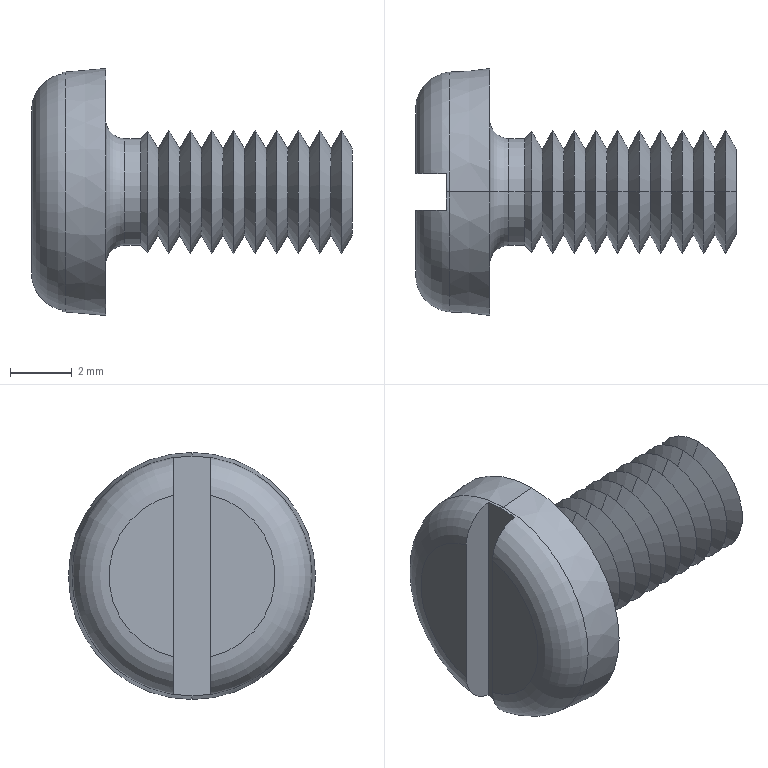Part | SolidWorks | features Cut 1, LPattern 1, RevCut 1, Revolution 1 | 1 solid | 55 faces | box 10.4 x 8 x 8 mm | volume 174.956 mm3 | cone 42 | plane 7 | torus 4 | cylinder 2 | commonest cylinder face diameters 3.464 x2
STEP:
#1=CARTESIAN_POINT('',(3.532,0.,1.732));
#2=VERTEX_POINT('',#1);
#3=CARTESIAN_POINT('',(3.532,0.,-1.732));
#4=VERTEX_POINT('',#3);
#5=CARTESIAN_POINT('',(3.532,0.,0.));
#6=DIRECTION('',(-1.,0.,0.));
#7=DIRECTION('',(0.,0.,1.));
#8=AXIS2_PLACEMENT_3D('',#5,#6,#7);
#9=CIRCLE('',#8,1.732);
#10=EDGE_CURVE('',#2,#4,#9,.T.);
#11=ORIENTED_EDGE('',*,*,#10,.F.);
#12=CARTESIAN_POINT('',(3.766,0.,1.966));
#13=VERTEX_POINT('',#12);
#14=CARTESIAN_POINT('',(3.8,0.,2.));
#15=DIRECTION('',(0.7071,0.,0.7071));
#16=VECTOR('',#15,1000.);
#17=LINE('',#14,#16);
#18=EDGE_CURVE('',#2,#13,#17,.T.);
#19=ORIENTED_EDGE('',*,*,#18,.T.);
#20=CARTESIAN_POINT('',(3.766,0.,-1.966));
#21=VERTEX_POINT('',#20);
#22=CARTESIAN_POINT('',(3.766,0.,0.));
#23=DIRECTION('',(-1.,0.,0.));
#24=DIRECTION('',(0.,0.,1.));
#25=AXIS2_PLACEMENT_3D('',#22,#23,#24);
#26=CIRCLE('',#25,1.966);
#27=EDGE_CURVE('',#13,#21,#26,.T.);
#28=ORIENTED_EDGE('',*,*,#27,.T.);
#29=CARTESIAN_POINT('',(3.8,0.,-2.));
#30=DIRECTION('',(0.7071,0.,-0.7071));
#31=VECTOR('',#30,1000.);
#32=LINE('',#29,#31);
#33=EDGE_CURVE('',#4,#21,#32,.T.);
#34=ORIENTED_EDGE('',*,*,#33,.F.);
#35=EDGE_LOOP('',(#11,#19,#28,#34));
#36=FACE_OUTER_BOUND('',#35,.T.);
#37=CARTESIAN_POINT('',(3.8,0.,0.));
#38=DIRECTION('',(1.,0.,0.));
#39=DIRECTION('',(0.,0.,-1.));
#40=AXIS2_PLACEMENT_3D('',#37,#38,#39);
#41=CONICAL_SURFACE('',#40,2.,0.7854);
#42=ADVANCED_FACE('',(#36),#41,.T.);
#43=ORIENTED_EDGE('',*,*,#10,.T.);
#44=CARTESIAN_POINT('',(3.018,0.,-1.732));
#45=VERTEX_POINT('',#44);
#46=CARTESIAN_POINT('',(-2.477,0.,-1.732));
#47=DIRECTION('',(-1.,0.,0.));
#48=VECTOR('',#47,1000.);
#49=LINE('',#46,#48);
#50=EDGE_CURVE('',#4,#45,#49,.T.);
#51=ORIENTED_EDGE('',*,*,#50,.T.);
#52=CARTESIAN_POINT('',(3.018,0.,1.732));
#53=VERTEX_POINT('',#52);
#54=CARTESIAN_POINT('',(3.018,0.,0.));
#55=DIRECTION('',(-1.,0.,0.));
#56=DIRECTION('',(0.,0.,1.));
#57=AXIS2_PLACEMENT_3D('',#54,#55,#56);
#58=CIRCLE('',#57,1.732);
#59=EDGE_CURVE('',#53,#45,#58,.T.);
#60=ORIENTED_EDGE('',*,*,#59,.F.);
#61=CARTESIAN_POINT('',(-2.477,0.,1.732));
#62=DIRECTION('',(-1.,0.,0.));
#63=VECTOR('',#62,1000.);
#64=LINE('',#61,#63);
#65=EDGE_CURVE('',#2,#53,#64,.T.);
#66=ORIENTED_EDGE('',*,*,#65,.F.);
#67=EDGE_LOOP('',(#43,#51,#60,#66));
#68=FACE_OUTER_BOUND('',#67,.T.);
#69=CARTESIAN_POINT('',(-2.477,0.,0.));
#70=DIRECTION('',(-1.,0.,0.));
#71=DIRECTION('',(0.,0.,1.));
#72=AXIS2_PLACEMENT_3D('',#69,#70,#71);
#73=CYLINDRICAL_SURFACE('',#72,1.732);
#74=ADVANCED_FACE('',(#68),#73,.T.);
#75=CARTESIAN_POINT('',(2.4,0.,-2.35));
#76=VERTEX_POINT('',#75);
#77=CARTESIAN_POINT('',(2.4,0.,2.35));
#78=VERTEX_POINT('',#77);
#79=CARTESIAN_POINT('',(2.4,0.,0.));
#80=DIRECTION('',(-1.,0.,0.));
#81=DIRECTION('',(0.,0.,1.));
#82=AXIS2_PLACEMENT_3D('',#79,#80,#81);
#83=CIRCLE('',#82,2.35);
#84=EDGE_CURVE('',#76,#78,#83,.T.);
#85=ORIENTED_EDGE('',*,*,#84,.F.);
#86=CARTESIAN_POINT('',(3.018,0.,-2.35));
#87=DIRECTION('',(0.,1.,0.));
#88=DIRECTION('',(0.,0.,1.));
#89=AXIS2_PLACEMENT_3D('',#86,#87,#88);
#90=CIRCLE('',#89,0.618);
#91=EDGE_CURVE('',#76,#45,#90,.T.);
#92=ORIENTED_EDGE('',*,*,#91,.T.);
#93=CARTESIAN_POINT('',(3.018,0.,0.));
#94=DIRECTION('',(-1.,0.,0.));
#95=DIRECTION('',(0.,0.,1.));
#96=AXIS2_PLACEMENT_3D('',#93,#94,#95);
#97=CIRCLE('',#96,1.732);
#98=EDGE_CURVE('',#45,#53,#97,.T.);
#99=ORIENTED_EDGE('',*,*,#98,.T.);
#100=CARTESIAN_POINT('',(3.018,0.,2.35));
#101=DIRECTION('',(0.,-1.,0.));
#102=DIRECTION('',(0.,0.,-1.));
#103=AXIS2_PLACEMENT_3D('',#100,#101,#102);
#104=CIRCLE('',#103,0.618);
#105=EDGE_CURVE('',#78,#53,#104,.T.);
#106=ORIENTED_EDGE('',*,*,#105,.F.);
#107=EDGE_LOOP('',(#85,#92,#99,#106));
#108=FACE_OUTER_BOUND('',#107,.T.);
#109=CARTESIAN_POINT('',(3.018,0.,0.));
#110=DIRECTION('',(-1.,0.,0.));
#111=DIRECTION('',(0.,0.,1.));
#112=AXIS2_PLACEMENT_3D('',#109,#110,#111);
#113=TOROIDAL_SURFACE('',#112,2.35,0.618);
#114=ADVANCED_FACE('',(#108),#113,.F.);
#115=CARTESIAN_POINT('',(1.095,0.,3.886));
#116=VERTEX_POINT('',#115);
#117=CARTESIAN_POINT('',(1.095,0.,-3.886));
#118=VERTEX_POINT('',#117);
#119=CARTESIAN_POINT('',(1.095,0.,0.));
#120=DIRECTION('',(-1.,0.,0.));
#121=DIRECTION('',(0.,0.,1.));
#122=AXIS2_PLACEMENT_3D('',#119,#120,#121);
#123=CIRCLE('',#122,3.886);
#124=EDGE_CURVE('',#116,#118,#123,.T.);
#125=ORIENTED_EDGE('',*,*,#124,.F.);
#126=CARTESIAN_POINT('',(2.4,0.,4.));
#127=VERTEX_POINT('',#126);
#128=CARTESIAN_POINT('',(2.4,0.,4.));
#129=DIRECTION('',(0.9962,0.,0.08716));
#130=VECTOR('',#129,1000.);
#131=LINE('',#128,#130);
#132=EDGE_CURVE('',#116,#127,#131,.T.);
#133=ORIENTED_EDGE('',*,*,#132,.T.);
#134=CARTESIAN_POINT('',(2.4,0.,-4.));
#135=VERTEX_POINT('',#134);
#136=CARTESIAN_POINT('',(2.4,0.,0.));
#137=DIRECTION('',(-1.,0.,0.));
#138=DIRECTION('',(0.,0.,1.));
#139=AXIS2_PLACEMENT_3D('',#136,#137,#138);
#140=CIRCLE('',#139,4.);
#141=EDGE_CURVE('',#127,#135,#140,.T.);
#142=ORIENTED_EDGE('',*,*,#141,.T.);
#143=CARTESIAN_POINT('',(2.4,0.,-4.));
#144=DIRECTION('',(0.9962,0.,-0.08716));
#145=VECTOR('',#144,1000.);
#146=LINE('',#143,#145);
#147=EDGE_CURVE('',#118,#135,#146,.T.);
#148=ORIENTED_EDGE('',*,*,#147,.F.);
#149=EDGE_LOOP('',(#125,#133,#142,#148));
#150=FACE_OUTER_BOUND('',#149,.T.);
#151=CARTESIAN_POINT('',(2.4,0.,0.));
#152=DIRECTION('',(1.,0.,0.));
#153=DIRECTION('',(0.,0.,-1.));
#154=AXIS2_PLACEMENT_3D('',#151,#152,#153);
#155=CONICAL_SURFACE('',#154,4.,0.08727);
#156=ADVANCED_FACE('',(#150),#155,.T.);
#157=ORIENTED_EDGE('',*,*,#124,.T.);
#158=CARTESIAN_POINT('',(1.,0.,-3.874));
#159=VERTEX_POINT('',#158);
#160=CARTESIAN_POINT('',(1.2,0.,-2.69));
#161=DIRECTION('',(0.,1.,0.));
#162=DIRECTION('',(0.,0.,1.));
#163=AXIS2_PLACEMENT_3D('',#160,#161,#162);
#164=CIRCLE('',#163,1.2);
#165=EDGE_CURVE('',#118,#159,#164,.T.);
#166=ORIENTED_EDGE('',*,*,#165,.T.);
#167=CARTESIAN_POINT('',(1.,0.6,-3.827));
#168=VERTEX_POINT('',#167);
#169=CARTESIAN_POINT('',(1.,0.,0.));
#170=DIRECTION('',(1.,0.,0.));
#171=DIRECTION('',(0.,1.,0.));
#172=AXIS2_PLACEMENT_3D('',#169,#170,#171);
#173=CIRCLE('',#172,3.874);
#174=EDGE_CURVE('',#159,#168,#173,.T.);
#175=ORIENTED_EDGE('',*,*,#174,.T.);
#176=CARTESIAN_POINT('',(0.,0.6,-2.623));
#177=VERTEX_POINT('',#176);
#178=CARTESIAN_POINT('',(1.,0.6,-3.827));
#179=CARTESIAN_POINT('',(0.86,0.6,-3.803));
#180=CARTESIAN_POINT('',(0.7256,0.6,-3.754));
#181=CARTESIAN_POINT('',(0.4794,0.6,-3.611));
#182=CARTESIAN_POINT('',(0.3687,0.6,-3.516));
#183=CARTESIAN_POINT('',(0.1895,0.6,-3.298));
#184=CARTESIAN_POINT('',(0.1184,0.6,-3.172));
#185=CARTESIAN_POINT('',(0.02425,0.6,-2.906));
#186=CARTESIAN_POINT('',(0.,0.6,-2.764));
#187=CARTESIAN_POINT('',(0.,0.6,-2.623));
#188=B_SPLINE_CURVE_WITH_KNOTS('',3,(#178,#179,#180,#181,#182,#183,#184,#185,#186,#187),.UNSPECIFIED.,.F.,.F.,(4,2,2,2,4),(0.006929,0.007352,0.007774,0.008197,0.00862),.UNSPECIFIED.);
#189=EDGE_CURVE('',#168,#177,#188,.T.);
#190=ORIENTED_EDGE('',*,*,#189,.T.);
#191=CARTESIAN_POINT('',(0.,0.6,2.623));
#192=VERTEX_POINT('',#191);
#193=CARTESIAN_POINT('',(0.,0.,0.));
#194=DIRECTION('',(-1.,0.,0.));
#195=DIRECTION('',(0.,0.,1.));
#196=AXIS2_PLACEMENT_3D('',#193,#194,#195);
#197=CIRCLE('',#196,2.69);
#198=EDGE_CURVE('',#192,#177,#197,.T.);
#199=ORIENTED_EDGE('',*,*,#198,.F.);
#200=CARTESIAN_POINT('',(1.,0.6,3.827));
#201=VERTEX_POINT('',#200);
#202=CARTESIAN_POINT('',(0.,0.6,2.623));
#203=CARTESIAN_POINT('',(0.,0.6,2.908));
#204=CARTESIAN_POINT('',(0.09837,0.6,3.188));
#205=CARTESIAN_POINT('',(0.3703,0.6,3.518));
#206=CARTESIAN_POINT('',(0.4787,0.6,3.61));
#207=CARTESIAN_POINT('',(0.7255,0.6,3.754));
#208=CARTESIAN_POINT('',(0.8588,0.6,3.803));
#209=CARTESIAN_POINT('',(1.,0.6,3.827));
#210=B_SPLINE_CURVE_WITH_KNOTS('',3,(#202,#203,#204,#205,#206,#207,#208,#209),.UNSPECIFIED.,.F.,.F.,(4,2,2,4),(0.001251,0.002097,0.00252,0.002944),.UNSPECIFIED.);
#211=EDGE_CURVE('',#192,#201,#210,.T.);
#212=ORIENTED_EDGE('',*,*,#211,.T.);
#213=CARTESIAN_POINT('',(1.,0.,3.874));
#214=VERTEX_POINT('',#213);
#215=CARTESIAN_POINT('',(1.,0.,0.));
#216=DIRECTION('',(1.,0.,0.));
#217=DIRECTION('',(0.,1.,0.));
#218=AXIS2_PLACEMENT_3D('',#215,#216,#217);
#219=CIRCLE('',#218,3.874);
#220=EDGE_CURVE('',#201,#214,#219,.T.);
#221=ORIENTED_EDGE('',*,*,#220,.T.);
#222=CARTESIAN_POINT('',(1.2,0.,2.69));
#223=DIRECTION('',(0.,-1.,0.));
#224=DIRECTION('',(0.,0.,-1.));
#225=AXIS2_PLACEMENT_3D('',#222,#223,#224);
#226=CIRCLE('',#225,1.2);
#227=EDGE_CURVE('',#116,#214,#226,.T.);
#228=ORIENTED_EDGE('',*,*,#227,.F.);
#229=EDGE_LOOP('',(#157,#166,#175,#190,#199,#212,#221,#228));
#230=FACE_OUTER_BOUND('',#229,.T.);
#231=CARTESIAN_POINT('',(1.2,0.,0.));
#232=DIRECTION('',(-1.,0.,0.));
#233=DIRECTION('',(0.,0.,1.));
#234=AXIS2_PLACEMENT_3D('',#231,#232,#233);
#235=TOROIDAL_SURFACE('',#234,2.69,1.2);
#236=ADVANCED_FACE('',(#230),#235,.T.);
#237=CARTESIAN_POINT('',(4.1,0.,-1.394));
#238=VERTEX_POINT('',#237);
#239=CARTESIAN_POINT('',(4.1,0.,1.394));
#240=VERTEX_POINT('',#239);
#241=CARTESIAN_POINT('',(4.1,0.,0.));
#242=DIRECTION('',(1.,0.,0.));
#243=DIRECTION('',(0.,0.,-1.));
#244=AXIS2_PLACEMENT_3D('',#241,#242,#243);
#245=CIRCLE('',#244,1.394);
#246=EDGE_CURVE('',#238,#240,#245,.T.);
#247=ORIENTED_EDGE('',*,*,#246,.T.);
#248=CARTESIAN_POINT('',(4.446,0.,2.));
#249=VERTEX_POINT('',#248);
#250=CARTESIAN_POINT('',(4.1,0.,1.394));
#251=DIRECTION('',(0.4959,0.,0.8684));
#252=VECTOR('',#251,1000.);
#253=LINE('',#250,#252);
#254=EDGE_CURVE('',#240,#249,#253,.T.);
#255=ORIENTED_EDGE('',*,*,#254,.T.);
#256=CARTESIAN_POINT('',(4.446,0.,-2.));
#257=VERTEX_POINT('',#256);
#258=CARTESIAN_POINT('',(4.446,0.,0.));
#259=DIRECTION('',(1.,0.,0.));
#260=DIRECTION('',(0.,0.,-1.));
#261=AXIS2_PLACEMENT_3D('',#258,#259,#260);
#262=CIRCLE('',#261,2.);
#263=EDGE_CURVE('',#257,#249,#262,.T.);
#264=ORIENTED_EDGE('',*,*,#263,.F.);
#265=CARTESIAN_POINT('',(4.1,0.,-1.394));
#266=DIRECTION('',(0.4959,0.,-0.8684));
#267=VECTOR('',#266,1000.);
#268=LINE('',#265,#267);
#269=EDGE_CURVE('',#238,#257,#268,.T.);
#270=ORIENTED_EDGE('',*,*,#269,.F.);
#271=EDGE_LOOP('',(#247,#255,#264,#270));
#272=FACE_OUTER_BOUND('',#271,.T.);
#273=CARTESIAN_POINT('',(4.1,0.,0.));
#274=DIRECTION('',(1.,0.,0.));
#275=DIRECTION('',(0.,0.,-1.));
#276=AXIS2_PLACEMENT_3D('',#273,#274,#275);
#277=CONICAL_SURFACE('',#276,1.394,1.052);
#278=ADVANCED_FACE('',(#272),#277,.T.);
#279=ORIENTED_EDGE('',*,*,#246,.F.);
#280=CARTESIAN_POINT('',(3.746,0.,-2.));
#281=DIRECTION('',(-0.5041,0.,-0.8637));
#282=VECTOR('',#281,1000.);
#283=LINE('',#280,#282);
#284=EDGE_CURVE('',#238,#21,#283,.T.);
#285=ORIENTED_EDGE('',*,*,#284,.T.);
#286=ORIENTED_EDGE('',*,*,#27,.F.);
#287=CARTESIAN_POINT('',(3.746,0.,2.));
#288=DIRECTION('',(-0.5041,0.,0.8637));
#289=VECTOR('',#288,1000.);
#290=LINE('',#287,#289);
#291=EDGE_CURVE('',#240,#13,#290,.T.);
#292=ORIENTED_EDGE('',*,*,#291,.F.);
#293=EDGE_LOOP('',(#279,#285,#286,#292));
#294=FACE_OUTER_BOUND('',#293,.T.);
#295=CARTESIAN_POINT('',(3.746,0.,0.));
#296=DIRECTION('',(-1.,0.,0.));
#297=DIRECTION('',(0.,0.,1.));
#298=AXIS2_PLACEMENT_3D('',#295,#296,#297);
#299=CONICAL_SURFACE('',#298,2.,1.043);
#300=ADVANCED_FACE('',(#294),#299,.T.);
#301=CARTESIAN_POINT('',(4.8,0.,-1.394));
#302=VERTEX_POINT('',#301);
#303=CARTESIAN_POINT('',(4.8,0.,1.394));
#304=VERTEX_POINT('',#303);
#305=CARTESIAN_POINT('',(4.8,0.,0.));
#306=DIRECTION('',(1.,0.,0.));
#307=DIRECTION('',(0.,0.,-1.));
#308=AXIS2_PLACEMENT_3D('',#305,#306,#307);
#309=CIRCLE('',#308,1.394);
#310=EDGE_CURVE('',#302,#304,#309,.T.);
#311=ORIENTED_EDGE('',*,*,#310,.T.);
#312=CARTESIAN_POINT('',(5.146,0.,2.));
#313=VERTEX_POINT('',#312);
#314=CARTESIAN_POINT('',(4.8,0.,1.394));
#315=DIRECTION('',(0.4959,0.,0.8684));
#316=VECTOR('',#315,1000.);
#317=LINE('',#314,#316);
#318=EDGE_CURVE('',#304,#313,#317,.T.);
#319=ORIENTED_EDGE('',*,*,#318,.T.);
#320=CARTESIAN_POINT('',(5.146,0.,-2.));
#321=VERTEX_POINT('',#320);
#322=CARTESIAN_POINT('',(5.146,0.,0.));
#323=DIRECTION('',(1.,0.,0.));
#324=DIRECTION('',(0.,0.,-1.));
#325=AXIS2_PLACEMENT_3D('',#322,#323,#324);
#326=CIRCLE('',#325,2.);
#327=EDGE_CURVE('',#321,#313,#326,.T.);
#328=ORIENTED_EDGE('',*,*,#327,.F.);
#329=CARTESIAN_POINT('',(4.8,0.,-1.394));
#330=DIRECTION('',(0.4959,0.,-0.8684));
#331=VECTOR('',#330,1000.);
#332=LINE('',#329,#331);
#333=EDGE_CURVE('',#302,#321,#332,.T.);
#334=ORIENTED_EDGE('',*,*,#333,.F.);
#335=EDGE_LOOP('',(#311,#319,#328,#334));
#336=FACE_OUTER_BOUND('',#335,.T.);
#337=CARTESIAN_POINT('',(4.8,0.,0.));
#338=DIRECTION('',(1.,0.,0.));
#339=DIRECTION('',(0.,0.,-1.));
#340=AXIS2_PLACEMENT_3D('',#337,#338,#339);
#341=CONICAL_SURFACE('',#340,1.394,1.052);
#342=ADVANCED_FACE('',(#336),#341,.T.);
#343=ORIENTED_EDGE('',*,*,#310,.F.);
#344=CARTESIAN_POINT('',(4.446,0.,-2.));
#345=DIRECTION('',(-0.5041,0.,-0.8637));
#346=VECTOR('',#345,1000.);
#347=LINE('',#344,#346);
#348=EDGE_CURVE('',#302,#257,#347,.T.);
#349=ORIENTED_EDGE('',*,*,#348,.T.);
#350=ORIENTED_EDGE('',*,*,#263,.T.);
#351=CARTESIAN_POINT('',(4.446,0.,2.));
#352=DIRECTION('',(-0.5041,0.,0.8637));
#353=VECTOR('',#352,1000.);
#354=LINE('',#351,#353);
#355=EDGE_CURVE('',#304,#249,#354,.T.);
#356=ORIENTED_EDGE('',*,*,#355,.F.);
#357=EDGE_LOOP('',(#343,#349,#350,#356));
#358=FACE_OUTER_BOUND('',#357,.T.);
#359=CARTESIAN_POINT('',(4.446,0.,0.));
#360=DIRECTION('',(-1.,0.,0.));
#361=DIRECTION('',(0.,0.,1.));
#362=AXIS2_PLACEMENT_3D('',#359,#360,#361);
#363=CONICAL_SURFACE('',#362,2.,1.043);
#364=ADVANCED_FACE('',(#358),#363,.T.);
#365=CARTESIAN_POINT('',(5.5,0.,-1.394));
#366=VERTEX_POINT('',#365);
#367=CARTESIAN_POINT('',(5.5,0.,1.394));
#368=VERTEX_POINT('',#367);
#369=CARTESIAN_POINT('',(5.5,0.,0.));
#370=DIRECTION('',(1.,0.,0.));
#371=DIRECTION('',(0.,0.,-1.));
#372=AXIS2_PLACEMENT_3D('',#369,#370,#371);
#373=CIRCLE('',#372,1.394);
#374=EDGE_CURVE('',#366,#368,#373,.T.);
#375=ORIENTED_EDGE('',*,*,#374,.T.);
#376=CARTESIAN_POINT('',(5.846,0.,2.));
#377=VERTEX_POINT('',#376);
#378=CARTESIAN_POINT('',(5.5,0.,1.394));
#379=DIRECTION('',(0.4959,0.,0.8684));
#380=VECTOR('',#379,1000.);
#381=LINE('',#378,#380);
#382=EDGE_CURVE('',#368,#377,#381,.T.);
#383=ORIENTED_EDGE('',*,*,#382,.T.);
#384=CARTESIAN_POINT('',(5.846,0.,-2.));
#385=VERTEX_POINT('',#384);
#386=CARTESIAN_POINT('',(5.846,0.,0.));
#387=DIRECTION('',(1.,0.,0.));
#388=DIRECTION('',(0.,0.,-1.));
#389=AXIS2_PLACEMENT_3D('',#386,#387,#388);
#390=CIRCLE('',#389,2.);
#391=EDGE_CURVE('',#385,#377,#390,.T.);
#392=ORIENTED_EDGE('',*,*,#391,.F.);
#393=CARTESIAN_POINT('',(5.5,0.,-1.394));
#394=DIRECTION('',(0.4959,0.,-0.8684));
#395=VECTOR('',#394,1000.);
#396=LINE('',#393,#395);
#397=EDGE_CURVE('',#366,#385,#396,.T.);
#398=ORIENTED_EDGE('',*,*,#397,.F.);
#399=EDGE_LOOP('',(#375,#383,#392,#398));
#400=FACE_OUTER_BOUND('',#399,.T.);
#401=CARTESIAN_POINT('',(5.5,0.,0.));
#402=DIRECTION('',(1.,0.,0.));
#403=DIRECTION('',(0.,0.,-1.));
#404=AXIS2_PLACEMENT_3D('',#401,#402,#403);
#405=CONICAL_SURFACE('',#404,1.394,1.052);
#406=ADVANCED_FACE('',(#400),#405,.T.);
#407=ORIENTED_EDGE('',*,*,#374,.F.);
#408=CARTESIAN_POINT('',(5.146,0.,-2.));
#409=DIRECTION('',(-0.5041,0.,-0.8637));
#410=VECTOR('',#409,1000.);
#411=LINE('',#408,#410);
#412=EDGE_CURVE('',#366,#321,#411,.T.);
#413=ORIENTED_EDGE('',*,*,#412,.T.);
#414=ORIENTED_EDGE('',*,*,#327,.T.);
#415=CARTESIAN_POINT('',(5.146,0.,2.));
#416=DIRECTION('',(-0.5041,0.,0.8637));
#417=VECTOR('',#416,1000.);
#418=LINE('',#415,#417);
#419=EDGE_CURVE('',#368,#313,#418,.T.);
#420=ORIENTED_EDGE('',*,*,#419,.F.);
#421=EDGE_LOOP('',(#407,#413,#414,#420));
#422=FACE_OUTER_BOUND('',#421,.T.);
#423=CARTESIAN_POINT('',(5.146,0.,0.));
#424=DIRECTION('',(-1.,0.,0.));
#425=DIRECTION('',(0.,0.,1.));
#426=AXIS2_PLACEMENT_3D('',#423,#424,#425);
#427=CONICAL_SURFACE('',#426,2.,1.043);
#428=ADVANCED_FACE('',(#422),#427,.T.);
#429=CARTESIAN_POINT('',(6.2,0.,-1.394));
#430=VERTEX_POINT('',#429);
#431=CARTESIAN_POINT('',(6.2,0.,1.394));
#432=VERTEX_POINT('',#431);
#433=CARTESIAN_POINT('',(6.2,0.,0.));
#434=DIRECTION('',(1.,0.,0.));
#435=DIRECTION('',(0.,0.,-1.));
#436=AXIS2_PLACEMENT_3D('',#433,#434,#435);
#437=CIRCLE('',#436,1.394);
#438=EDGE_CURVE('',#430,#432,#437,.T.);
#439=ORIENTED_EDGE('',*,*,#438,.T.);
#440=CARTESIAN_POINT('',(6.546,0.,2.));
#441=VERTEX_POINT('',#440);
#442=CARTESIAN_POINT('',(6.2,0.,1.394));
#443=DIRECTION('',(0.4959,0.,0.8684));
#444=VECTOR('',#443,1000.);
#445=LINE('',#442,#444);
#446=EDGE_CURVE('',#432,#441,#445,.T.);
#447=ORIENTED_EDGE('',*,*,#446,.T.);
#448=CARTESIAN_POINT('',(6.546,0.,-2.));
#449=VERTEX_POINT('',#448);
#450=CARTESIAN_POINT('',(6.546,0.,0.));
#451=DIRECTION('',(1.,0.,0.));
#452=DIRECTION('',(0.,0.,-1.));
#453=AXIS2_PLACEMENT_3D('',#450,#451,#452);
#454=CIRCLE('',#453,2.);
#455=EDGE_CURVE('',#449,#441,#454,.T.);
#456=ORIENTED_EDGE('',*,*,#455,.F.);
#457=CARTESIAN_POINT('',(6.2,0.,-1.394));
#458=DIRECTION('',(0.4959,0.,-0.8684));
#459=VECTOR('',#458,1000.);
#460=LINE('',#457,#459);
#461=EDGE_CURVE('',#430,#449,#460,.T.);
#462=ORIENTED_EDGE('',*,*,#461,.F.);
#463=EDGE_LOOP('',(#439,#447,#456,#462));
#464=FACE_OUTER_BOUND('',#463,.T.);
#465=CARTESIAN_POINT('',(6.2,0.,0.));
#466=DIRECTION('',(1.,0.,0.));
#467=DIRECTION('',(0.,0.,-1.));
#468=AXIS2_PLACEMENT_3D('',#465,#466,#467);
#469=CONICAL_SURFACE('',#468,1.394,1.052);
#470=ADVANCED_FACE('',(#464),#469,.T.);
#471=ORIENTED_EDGE('',*,*,#438,.F.);
#472=CARTESIAN_POINT('',(5.846,0.,-2.));
#473=DIRECTION('',(-0.5041,0.,-0.8637));
#474=VECTOR('',#473,1000.);
#475=LINE('',#472,#474);
#476=EDGE_CURVE('',#430,#385,#475,.T.);
#477=ORIENTED_EDGE('',*,*,#476,.T.);
#478=ORIENTED_EDGE('',*,*,#391,.T.);
#479=CARTESIAN_POINT('',(5.846,0.,2.));
#480=DIRECTION('',(-0.5041,0.,0.8637));
#481=VECTOR('',#480,1000.);
#482=LINE('',#479,#481);
#483=EDGE_CURVE('',#432,#377,#482,.T.);
#484=ORIENTED_EDGE('',*,*,#483,.F.);
#485=EDGE_LOOP('',(#471,#477,#478,#484));
#486=FACE_OUTER_BOUND('',#485,.T.);
#487=CARTESIAN_POINT('',(5.846,0.,0.));
#488=DIRECTION('',(-1.,0.,0.));
#489=DIRECTION('',(0.,0.,1.));
#490=AXIS2_PLACEMENT_3D('',#487,#488,#489);
#491=CONICAL_SURFACE('',#490,2.,1.043);
#492=ADVANCED_FACE('',(#486),#491,.T.);
#493=CARTESIAN_POINT('',(6.9,0.,-1.394));
#494=VERTEX_POINT('',#493);
#495=CARTESIAN_POINT('',(6.9,0.,1.394));
#496=VERTEX_POINT('',#495);
#497=CARTESIAN_POINT('',(6.9,0.,0.));
#498=DIRECTION('',(1.,0.,0.));
#499=DIRECTION('',(0.,0.,-1.));
#500=AXIS2_PLACEMENT_3D('',#497,#498,#499);
#501=CIRCLE('',#500,1.394);
#502=EDGE_CURVE('',#494,#496,#501,.T.);
#503=ORIENTED_EDGE('',*,*,#502,.T.);
#504=CARTESIAN_POINT('',(7.246,0.,2.));
#505=VERTEX_POINT('',#504);
#506=CARTESIAN_POINT('',(6.9,0.,1.394));
#507=DIRECTION('',(0.4959,0.,0.8684));
#508=VECTOR('',#507,1000.);
#509=LINE('',#506,#508);
#510=EDGE_CURVE('',#496,#505,#509,.T.);
#511=ORIENTED_EDGE('',*,*,#510,.T.);
#512=CARTESIAN_POINT('',(7.246,0.,-2.));
#513=VERTEX_POINT('',#512);
#514=CARTESIAN_POINT('',(7.246,0.,0.));
#515=DIRECTION('',(1.,0.,0.));
#516=DIRECTION('',(0.,0.,-1.));
#517=AXIS2_PLACEMENT_3D('',#514,#515,#516);
#518=CIRCLE('',#517,2.);
#519=EDGE_CURVE('',#513,#505,#518,.T.);
#520=ORIENTED_EDGE('',*,*,#519,.F.);
#521=CARTESIAN_POINT('',(6.9,0.,-1.394));
#522=DIRECTION('',(0.4959,0.,-0.8684));
#523=VECTOR('',#522,1000.);
#524=LINE('',#521,#523);
#525=EDGE_CURVE('',#494,#513,#524,.T.);
#526=ORIENTED_EDGE('',*,*,#525,.F.);
#527=EDGE_LOOP('',(#503,#511,#520,#526));
#528=FACE_OUTER_BOUND('',#527,.T.);
#529=CARTESIAN_POINT('',(6.9,0.,0.));
#530=DIRECTION('',(1.,0.,0.));
#531=DIRECTION('',(0.,0.,-1.));
#532=AXIS2_PLACEMENT_3D('',#529,#530,#531);
#533=CONICAL_SURFACE('',#532,1.394,1.052);
#534=ADVANCED_FACE('',(#528),#533,.T.);
#535=ORIENTED_EDGE('',*,*,#502,.F.);
#536=CARTESIAN_POINT('',(6.546,0.,-2.));
#537=DIRECTION('',(-0.5041,0.,-0.8637));
#538=VECTOR('',#537,1000.);
#539=LINE('',#536,#538);
#540=EDGE_CURVE('',#494,#449,#539,.T.);
#541=ORIENTED_EDGE('',*,*,#540,.T.);
#542=ORIENTED_EDGE('',*,*,#455,.T.);
#543=CARTESIAN_POINT('',(6.546,0.,2.));
#544=DIRECTION('',(-0.5041,0.,0.8637));
#545=VECTOR('',#544,1000.);
#546=LINE('',#543,#545);
#547=EDGE_CURVE('',#496,#441,#546,.T.);
#548=ORIENTED_EDGE('',*,*,#547,.F.);
#549=EDGE_LOOP('',(#535,#541,#542,#548));
#550=FACE_OUTER_BOUND('',#549,.T.);
#551=CARTESIAN_POINT('',(6.546,0.,0.));
#552=DIRECTION('',(-1.,0.,0.));
#553=DIRECTION('',(0.,0.,1.));
#554=AXIS2_PLACEMENT_3D('',#551,#552,#553);
#555=CONICAL_SURFACE('',#554,2.,1.043);
#556=ADVANCED_FACE('',(#550),#555,.T.);
#557=CARTESIAN_POINT('',(8.3,0.,-1.394));
#558=VERTEX_POINT('',#557);
#559=CARTESIAN_POINT('',(8.3,0.,1.394));
#560=VERTEX_POINT('',#559);
#561=CARTESIAN_POINT('',(8.3,0.,0.));
#562=DIRECTION('',(1.,0.,0.));
#563=DIRECTION('',(0.,0.,-1.));
#564=AXIS2_PLACEMENT_3D('',#561,#562,#563);
#565=CIRCLE('',#564,1.394);
#566=EDGE_CURVE('',#558,#560,#565,.T.);
#567=ORIENTED_EDGE('',*,*,#566,.F.);
#568=CARTESIAN_POINT('',(7.946,0.,-2.));
#569=VERTEX_POINT('',#568);
#570=CARTESIAN_POINT('',(7.946,0.,-2.));
#571=DIRECTION('',(-0.5041,0.,-0.8637));
#572=VECTOR('',#571,1000.);
#573=LINE('',#570,#572);
#574=EDGE_CURVE('',#558,#569,#573,.T.);
#575=ORIENTED_EDGE('',*,*,#574,.T.);
#576=CARTESIAN_POINT('',(7.946,0.,2.));
#577=VERTEX_POINT('',#576);
#578=CARTESIAN_POINT('',(7.946,0.,0.));
#579=DIRECTION('',(1.,0.,0.));
#580=DIRECTION('',(0.,0.,-1.));
#581=AXIS2_PLACEMENT_3D('',#578,#579,#580);
#582=CIRCLE('',#581,2.);
#583=EDGE_CURVE('',#569,#577,#582,.T.);
#584=ORIENTED_EDGE('',*,*,#583,.T.);
#585=CARTESIAN_POINT('',(7.946,0.,2.));
#586=DIRECTION('',(-0.5041,0.,0.8637));
#587=VECTOR('',#586,1000.);
#588=LINE('',#585,#587);
#589=EDGE_CURVE('',#560,#577,#588,.T.);
#590=ORIENTED_EDGE('',*,*,#589,.F.);
#591=EDGE_LOOP('',(#567,#575,#584,#590));
#592=FACE_OUTER_BOUND('',#591,.T.);
#593=CARTESIAN_POINT('',(7.946,0.,0.));
#594=DIRECTION('',(-1.,0.,0.));
#595=DIRECTION('',(0.,0.,1.));
#596=AXIS2_PLACEMENT_3D('',#593,#594,#595);
#597=CONICAL_SURFACE('',#596,2.,1.043);
#598=ADVANCED_FACE('',(#592),#597,.T.);
#599=ORIENTED_EDGE('',*,*,#566,.T.);
#600=CARTESIAN_POINT('',(8.646,0.,2.));
#601=VERTEX_POINT('',#600);
#602=CARTESIAN_POINT('',(8.3,0.,1.394));
#603=DIRECTION('',(0.4959,0.,0.8684));
#604=VECTOR('',#603,1000.);
#605=LINE('',#602,#604);
#606=EDGE_CURVE('',#560,#601,#605,.T.);
#607=ORIENTED_EDGE('',*,*,#606,.T.);
#608=CARTESIAN_POINT('',(8.646,0.,-2.));
#609=VERTEX_POINT('',#608);
#610=CARTESIAN_POINT('',(8.646,0.,0.));
#611=DIRECTION('',(1.,0.,0.));
#612=DIRECTION('',(0.,0.,-1.));
#613=AXIS2_PLACEMENT_3D('',#610,#611,#612);
#614=CIRCLE('',#613,2.);
#615=EDGE_CURVE('',#609,#601,#614,.T.);
#616=ORIENTED_EDGE('',*,*,#615,.F.);
#617=CARTESIAN_POINT('',(8.3,0.,-1.394));
#618=DIRECTION('',(0.4959,0.,-0.8684));
#619=VECTOR('',#618,1000.);
#620=LINE('',#617,#619);
#621=EDGE_CURVE('',#558,#609,#620,.T.);
#622=ORIENTED_EDGE('',*,*,#621,.F.);
#623=EDGE_LOOP('',(#599,#607,#616,#622));
#624=FACE_OUTER_BOUND('',#623,.T.);
#625=CARTESIAN_POINT('',(8.3,0.,0.));
#626=DIRECTION('',(1.,0.,0.));
#627=DIRECTION('',(0.,0.,-1.));
#628=AXIS2_PLACEMENT_3D('',#625,#626,#627);
#629=CONICAL_SURFACE('',#628,1.394,1.052);
#630=ADVANCED_FACE('',(#624),#629,.T.);
#631=CARTESIAN_POINT('',(9.,0.,-1.394));
#632=VERTEX_POINT('',#631);
#633=CARTESIAN_POINT('',(9.,0.,1.394));
#634=VERTEX_POINT('',#633);
#635=CARTESIAN_POINT('',(9.,0.,0.));
#636=DIRECTION('',(1.,0.,0.));
#637=DIRECTION('',(0.,0.,-1.));
#638=AXIS2_PLACEMENT_3D('',#635,#636,#637);
#639=CIRCLE('',#638,1.394);
#640=EDGE_CURVE('',#632,#634,#639,.T.);
#641=ORIENTED_EDGE('',*,*,#640,.F.);
#642=CARTESIAN_POINT('',(8.646,0.,-2.));
#643=DIRECTION('',(-0.5041,0.,-0.8637));
#644=VECTOR('',#643,1000.);
#645=LINE('',#642,#644);
#646=EDGE_CURVE('',#632,#609,#645,.T.);
#647=ORIENTED_EDGE('',*,*,#646,.T.);
#648=ORIENTED_EDGE('',*,*,#615,.T.);
#649=CARTESIAN_POINT('',(8.646,0.,2.));
#650=DIRECTION('',(-0.5041,0.,0.8637));
#651=VECTOR('',#650,1000.);
#652=LINE('',#649,#651);
#653=EDGE_CURVE('',#634,#601,#652,.T.);
#654=ORIENTED_EDGE('',*,*,#653,.F.);
#655=EDGE_LOOP('',(#641,#647,#648,#654));
#656=FACE_OUTER_BOUND('',#655,.T.);
#657=CARTESIAN_POINT('',(8.646,0.,0.));
#658=DIRECTION('',(-1.,0.,0.));
#659=DIRECTION('',(0.,0.,1.));
#660=AXIS2_PLACEMENT_3D('',#657,#658,#659);
#661=CONICAL_SURFACE('',#660,2.,1.043);
#662=ADVANCED_FACE('',(#656),#661,.T.);
#663=ORIENTED_EDGE('',*,*,#640,.T.);
#664=CARTESIAN_POINT('',(9.346,0.,2.));
#665=VERTEX_POINT('',#664);
#666=CARTESIAN_POINT('',(9.,0.,1.394));
#667=DIRECTION('',(0.4959,0.,0.8684));
#668=VECTOR('',#667,1000.);
#669=LINE('',#666,#668);
#670=EDGE_CURVE('',#634,#665,#669,.T.);
#671=ORIENTED_EDGE('',*,*,#670,.T.);
#672=CARTESIAN_POINT('',(9.346,0.,-2.));
#673=VERTEX_POINT('',#672);
#674=CARTESIAN_POINT('',(9.346,0.,0.));
#675=DIRECTION('',(1.,0.,0.));
#676=DIRECTION('',(0.,0.,-1.));
#677=AXIS2_PLACEMENT_3D('',#674,#675,#676);
#678=CIRCLE('',#677,2.);
#679=EDGE_CURVE('',#673,#665,#678,.T.);
#680=ORIENTED_EDGE('',*,*,#679,.F.);
#681=CARTESIAN_POINT('',(9.,0.,-1.394));
#682=DIRECTION('',(0.4959,0.,-0.8684));
#683=VECTOR('',#682,1000.);
#684=LINE('',#681,#683);
#685=EDGE_CURVE('',#632,#673,#684,.T.);
#686=ORIENTED_EDGE('',*,*,#685,.F.);
#687=EDGE_LOOP('',(#663,#671,#680,#686));
#688=FACE_OUTER_BOUND('',#687,.T.);
#689=CARTESIAN_POINT('',(9.,0.,0.));
#690=DIRECTION('',(1.,0.,0.));
#691=DIRECTION('',(0.,0.,-1.));
#692=AXIS2_PLACEMENT_3D('',#689,#690,#691);
#693=CONICAL_SURFACE('',#692,1.394,1.052);
#694=ADVANCED_FACE('',(#688),#693,.T.);
#695=CARTESIAN_POINT('',(9.7,0.,-1.394));
#696=VERTEX_POINT('',#695);
#697=CARTESIAN_POINT('',(9.7,0.,1.394));
#698=VERTEX_POINT('',#697);
#699=CARTESIAN_POINT('',(9.7,0.,0.));
#700=DIRECTION('',(1.,0.,0.));
#701=DIRECTION('',(0.,0.,-1.));
#702=AXIS2_PLACEMENT_3D('',#699,#700,#701);
#703=CIRCLE('',#702,1.394);
#704=EDGE_CURVE('',#696,#698,#703,.T.);
#705=ORIENTED_EDGE('',*,*,#704,.F.);
#706=CARTESIAN_POINT('',(9.346,0.,-2.));
#707=DIRECTION('',(-0.5041,0.,-0.8637));
#708=VECTOR('',#707,1000.);
#709=LINE('',#706,#708);
#710=EDGE_CURVE('',#696,#673,#709,.T.);
#711=ORIENTED_EDGE('',*,*,#710,.T.);
#712=ORIENTED_EDGE('',*,*,#679,.T.);
#713=CARTESIAN_POINT('',(9.346,0.,2.));
#714=DIRECTION('',(-0.5041,0.,0.8637));
#715=VECTOR('',#714,1000.);
#716=LINE('',#713,#715);
#717=EDGE_CURVE('',#698,#665,#716,.T.);
#718=ORIENTED_EDGE('',*,*,#717,.F.);
#719=EDGE_LOOP('',(#705,#711,#712,#718));
#720=FACE_OUTER_BOUND('',#719,.T.);
#721=CARTESIAN_POINT('',(9.346,0.,0.));
#722=DIRECTION('',(-1.,0.,0.));
#723=DIRECTION('',(0.,0.,1.));
#724=AXIS2_PLACEMENT_3D('',#721,#722,#723);
#725=CONICAL_SURFACE('',#724,2.,1.043);
#726=ADVANCED_FACE('',(#720),#725,.T.);
#727=ORIENTED_EDGE('',*,*,#704,.T.);
#728=CARTESIAN_POINT('',(10.046,0.,2.));
#729=VERTEX_POINT('',#728);
#730=CARTESIAN_POINT('',(9.7,0.,1.394));
#731=DIRECTION('',(0.4959,0.,0.8684));
#732=VECTOR('',#731,1000.);
#733=LINE('',#730,#732);
#734=EDGE_CURVE('',#698,#729,#733,.T.);
#735=ORIENTED_EDGE('',*,*,#734,.T.);
#736=CARTESIAN_POINT('',(10.046,0.,-2.));
#737=VERTEX_POINT('',#736);
#738=CARTESIAN_POINT('',(10.046,0.,0.));
#739=DIRECTION('',(1.,0.,0.));
#740=DIRECTION('',(0.,0.,-1.));
#741=AXIS2_PLACEMENT_3D('',#738,#739,#740);
#742=CIRCLE('',#741,2.);
#743=EDGE_CURVE('',#737,#729,#742,.T.);
#744=ORIENTED_EDGE('',*,*,#743,.F.);
#745=CARTESIAN_POINT('',(9.7,0.,-1.394));
#746=DIRECTION('',(0.4959,0.,-0.8684));
#747=VECTOR('',#746,1000.);
#748=LINE('',#745,#747);
#749=EDGE_CURVE('',#696,#737,#748,.T.);
#750=ORIENTED_EDGE('',*,*,#749,.F.);
#751=EDGE_LOOP('',(#727,#735,#744,#750));
#752=FACE_OUTER_BOUND('',#751,.T.);
#753=CARTESIAN_POINT('',(9.7,0.,0.));
#754=DIRECTION('',(1.,0.,0.));
#755=DIRECTION('',(0.,0.,-1.));
#756=AXIS2_PLACEMENT_3D('',#753,#754,#755);
#757=CONICAL_SURFACE('',#756,1.394,1.052);
#758=ADVANCED_FACE('',(#752),#757,.T.);
#759=CARTESIAN_POINT('',(10.4,0.,-1.394));
#760=VERTEX_POINT('',#759);
#761=CARTESIAN_POINT('',(10.4,0.,1.394));
#762=VERTEX_POINT('',#761);
#763=CARTESIAN_POINT('',(10.4,0.,0.));
#764=DIRECTION('',(1.,0.,0.));
#765=DIRECTION('',(0.,0.,-1.));
#766=AXIS2_PLACEMENT_3D('',#763,#764,#765);
#767=CIRCLE('',#766,1.394);
#768=EDGE_CURVE('',#760,#762,#767,.T.);
#769=ORIENTED_EDGE('',*,*,#768,.F.);
#770=CARTESIAN_POINT('',(10.046,0.,-2.));
#771=DIRECTION('',(-0.5041,0.,-0.8637));
#772=VECTOR('',#771,1000.);
#773=LINE('',#770,#772);
#774=EDGE_CURVE('',#760,#737,#773,.T.);
#775=ORIENTED_EDGE('',*,*,#774,.T.);
#776=ORIENTED_EDGE('',*,*,#743,.T.);
#777=CARTESIAN_POINT('',(10.046,0.,2.));
#778=DIRECTION('',(-0.5041,0.,0.8637));
#779=VECTOR('',#778,1000.);
#780=LINE('',#777,#779);
#781=EDGE_CURVE('',#762,#729,#780,.T.);
#782=ORIENTED_EDGE('',*,*,#781,.F.);
#783=EDGE_LOOP('',(#769,#775,#776,#782));
#784=FACE_OUTER_BOUND('',#783,.T.);
#785=CARTESIAN_POINT('',(10.046,0.,0.));
#786=DIRECTION('',(-1.,0.,0.));
#787=DIRECTION('',(0.,0.,1.));
#788=AXIS2_PLACEMENT_3D('',#785,#786,#787);
#789=CONICAL_SURFACE('',#788,2.,1.043);
#790=ADVANCED_FACE('',(#784),#789,.T.);
#791=CARTESIAN_POINT('',(7.6,0.,-1.394));
#792=VERTEX_POINT('',#791);
#793=CARTESIAN_POINT('',(7.6,0.,1.394));
#794=VERTEX_POINT('',#793);
#795=CARTESIAN_POINT('',(7.6,0.,0.));
#796=DIRECTION('',(1.,0.,0.));
#797=DIRECTION('',(0.,0.,-1.));
#798=AXIS2_PLACEMENT_3D('',#795,#796,#797);
#799=CIRCLE('',#798,1.394);
#800=EDGE_CURVE('',#792,#794,#799,.T.);
#801=ORIENTED_EDGE('',*,*,#800,.T.);
#802=CARTESIAN_POINT('',(7.6,0.,1.394));
#803=DIRECTION('',(0.4959,0.,0.8684));
#804=VECTOR('',#803,1000.);
#805=LINE('',#802,#804);
#806=EDGE_CURVE('',#794,#577,#805,.T.);
#807=ORIENTED_EDGE('',*,*,#806,.T.);
#808=ORIENTED_EDGE('',*,*,#583,.F.);
#809=CARTESIAN_POINT('',(7.6,0.,-1.394));
#810=DIRECTION('',(0.4959,0.,-0.8684));
#811=VECTOR('',#810,1000.);
#812=LINE('',#809,#811);
#813=EDGE_CURVE('',#792,#569,#812,.T.);
#814=ORIENTED_EDGE('',*,*,#813,.F.);
#815=EDGE_LOOP('',(#801,#807,#808,#814));
#816=FACE_OUTER_BOUND('',#815,.T.);
#817=CARTESIAN_POINT('',(7.6,0.,0.));
#818=DIRECTION('',(1.,0.,0.));
#819=DIRECTION('',(0.,0.,-1.));
#820=AXIS2_PLACEMENT_3D('',#817,#818,#819);
#821=CONICAL_SURFACE('',#820,1.394,1.052);
#822=ADVANCED_FACE('',(#816),#821,.T.);
#823=ORIENTED_EDGE('',*,*,#800,.F.);
#824=CARTESIAN_POINT('',(7.246,0.,-2.));
#825=DIRECTION('',(-0.5041,0.,-0.8637));
#826=VECTOR('',#825,1000.);
#827=LINE('',#824,#826);
#828=EDGE_CURVE('',#792,#513,#827,.T.);
#829=ORIENTED_EDGE('',*,*,#828,.T.);
#830=ORIENTED_EDGE('',*,*,#519,.T.);
#831=CARTESIAN_POINT('',(7.246,0.,2.));
#832=DIRECTION('',(-0.5041,0.,0.8637));
#833=VECTOR('',#832,1000.);
#834=LINE('',#831,#833);
#835=EDGE_CURVE('',#794,#505,#834,.T.);
#836=ORIENTED_EDGE('',*,*,#835,.F.);
#837=EDGE_LOOP('',(#823,#829,#830,#836));
#838=FACE_OUTER_BOUND('',#837,.T.);
#839=CARTESIAN_POINT('',(7.246,0.,0.));
#840=DIRECTION('',(-1.,0.,0.));
#841=DIRECTION('',(0.,0.,1.));
#842=AXIS2_PLACEMENT_3D('',#839,#840,#841);
#843=CONICAL_SURFACE('',#842,2.,1.043);
#844=ADVANCED_FACE('',(#838),#843,.T.);
#845=ORIENTED_EDGE('',*,*,#828,.F.);
#846=CARTESIAN_POINT('',(7.6,0.,0.));
#847=DIRECTION('',(1.,0.,0.));
#848=DIRECTION('',(0.,0.,-1.));
#849=AXIS2_PLACEMENT_3D('',#846,#847,#848);
#850=CIRCLE('',#849,1.394);
#851=EDGE_CURVE('',#794,#792,#850,.T.);
#852=ORIENTED_EDGE('',*,*,#851,.F.);
#853=ORIENTED_EDGE('',*,*,#835,.T.);
#854=CARTESIAN_POINT('',(7.246,0.,0.));
#855=DIRECTION('',(1.,0.,0.));
#856=DIRECTION('',(0.,0.,-1.));
#857=AXIS2_PLACEMENT_3D('',#854,#855,#856);
#858=CIRCLE('',#857,2.);
#859=EDGE_CURVE('',#505,#513,#858,.T.);
#860=ORIENTED_EDGE('',*,*,#859,.T.);
#861=EDGE_LOOP('',(#845,#852,#853,#860));
#862=FACE_OUTER_BOUND('',#861,.T.);
#863=CARTESIAN_POINT('',(7.246,0.,0.));
#864=DIRECTION('',(-1.,0.,0.));
#865=DIRECTION('',(0.,0.,1.));
#866=AXIS2_PLACEMENT_3D('',#863,#864,#865);
#867=CONICAL_SURFACE('',#866,2.,1.043);
#868=ADVANCED_FACE('',(#862),#867,.T.);
#869=ORIENTED_EDGE('',*,*,#806,.F.);
#870=ORIENTED_EDGE('',*,*,#851,.T.);
#871=ORIENTED_EDGE('',*,*,#813,.T.);
#872=CARTESIAN_POINT('',(7.946,0.,0.));
#873=DIRECTION('',(1.,0.,0.));
#874=DIRECTION('',(0.,0.,-1.));
#875=AXIS2_PLACEMENT_3D('',#872,#873,#874);
#876=CIRCLE('',#875,2.);
#877=EDGE_CURVE('',#577,#569,#876,.T.);
#878=ORIENTED_EDGE('',*,*,#877,.F.);
#879=EDGE_LOOP('',(#869,#870,#871,#878));
#880=FACE_OUTER_BOUND('',#879,.T.);
#881=CARTESIAN_POINT('',(7.6,0.,0.));
#882=DIRECTION('',(1.,0.,0.));
#883=DIRECTION('',(0.,0.,-1.));
#884=AXIS2_PLACEMENT_3D('',#881,#882,#883);
#885=CONICAL_SURFACE('',#884,1.394,1.052);
#886=ADVANCED_FACE('',(#880),#885,.T.);
#887=CARTESIAN_POINT('',(10.4,0.,0.));
#888=DIRECTION('',(1.,0.,0.));
#889=DIRECTION('',(0.,0.,-1.));
#890=AXIS2_PLACEMENT_3D('',#887,#888,#889);
#891=CIRCLE('',#890,1.394);
#892=EDGE_CURVE('',#762,#760,#891,.T.);
#893=ORIENTED_EDGE('',*,*,#892,.T.);
#894=ORIENTED_EDGE('',*,*,#768,.T.);
#895=EDGE_LOOP('',(#893,#894));
#896=FACE_OUTER_BOUND('',#895,.T.);
#897=CARTESIAN_POINT('',(10.4,0.,0.));
#898=DIRECTION('',(-1.,0.,0.));
#899=DIRECTION('',(0.,0.,1.));
#900=AXIS2_PLACEMENT_3D('',#897,#898,#899);
#901=PLANE('',#900);
#902=ADVANCED_FACE('',(#896),#901,.F.);
#903=ORIENTED_EDGE('',*,*,#774,.F.);
#904=ORIENTED_EDGE('',*,*,#892,.F.);
#905=ORIENTED_EDGE('',*,*,#781,.T.);
#906=CARTESIAN_POINT('',(10.046,0.,0.));
#907=DIRECTION('',(1.,0.,0.));
#908=DIRECTION('',(0.,0.,-1.));
#909=AXIS2_PLACEMENT_3D('',#906,#907,#908);
#910=CIRCLE('',#909,2.);
#911=EDGE_CURVE('',#729,#737,#910,.T.);
#912=ORIENTED_EDGE('',*,*,#911,.T.);
#913=EDGE_LOOP('',(#903,#904,#905,#912));
#914=FACE_OUTER_BOUND('',#913,.T.);
#915=CARTESIAN_POINT('',(10.046,0.,0.));
#916=DIRECTION('',(-1.,0.,0.));
#917=DIRECTION('',(0.,0.,1.));
#918=AXIS2_PLACEMENT_3D('',#915,#916,#917);
#919=CONICAL_SURFACE('',#918,2.,1.043);
#920=ADVANCED_FACE('',(#914),#919,.T.);
#921=ORIENTED_EDGE('',*,*,#734,.F.);
#922=CARTESIAN_POINT('',(9.7,0.,0.));
#923=DIRECTION('',(1.,0.,0.));
#924=DIRECTION('',(0.,0.,-1.));
#925=AXIS2_PLACEMENT_3D('',#922,#923,#924);
#926=CIRCLE('',#925,1.394);
#927=EDGE_CURVE('',#698,#696,#926,.T.);
#928=ORIENTED_EDGE('',*,*,#927,.T.);
#929=ORIENTED_EDGE('',*,*,#749,.T.);
#930=ORIENTED_EDGE('',*,*,#911,.F.);
#931=EDGE_LOOP('',(#921,#928,#929,#930));
#932=FACE_OUTER_BOUND('',#931,.T.);
#933=CARTESIAN_POINT('',(9.7,0.,0.));
#934=DIRECTION('',(1.,0.,0.));
#935=DIRECTION('',(0.,0.,-1.));
#936=AXIS2_PLACEMENT_3D('',#933,#934,#935);
#937=CONICAL_SURFACE('',#936,1.394,1.052);
#938=ADVANCED_FACE('',(#932),#937,.T.);
#939=ORIENTED_EDGE('',*,*,#710,.F.);
#940=ORIENTED_EDGE('',*,*,#927,.F.);
#941=ORIENTED_EDGE('',*,*,#717,.T.);
#942=CARTESIAN_POINT('',(9.346,0.,0.));
#943=DIRECTION('',(1.,0.,0.));
#944=DIRECTION('',(0.,0.,-1.));
#945=AXIS2_PLACEMENT_3D('',#942,#943,#944);
#946=CIRCLE('',#945,2.);
#947=EDGE_CURVE('',#665,#673,#946,.T.);
#948=ORIENTED_EDGE('',*,*,#947,.T.);
#949=EDGE_LOOP('',(#939,#940,#941,#948));
#950=FACE_OUTER_BOUND('',#949,.T.);
#951=CARTESIAN_POINT('',(9.346,0.,0.));
#952=DIRECTION('',(-1.,0.,0.));
#953=DIRECTION('',(0.,0.,1.));
#954=AXIS2_PLACEMENT_3D('',#951,#952,#953);
#955=CONICAL_SURFACE('',#954,2.,1.043);
#956=ADVANCED_FACE('',(#950),#955,.T.);
#957=ORIENTED_EDGE('',*,*,#670,.F.);
#958=CARTESIAN_POINT('',(9.,0.,0.));
#959=DIRECTION('',(1.,0.,0.));
#960=DIRECTION('',(0.,0.,-1.));
#961=AXIS2_PLACEMENT_3D('',#958,#959,#960);
#962=CIRCLE('',#961,1.394);
#963=EDGE_CURVE('',#634,#632,#962,.T.);
#964=ORIENTED_EDGE('',*,*,#963,.T.);
#965=ORIENTED_EDGE('',*,*,#685,.T.);
#966=ORIENTED_EDGE('',*,*,#947,.F.);
#967=EDGE_LOOP('',(#957,#964,#965,#966));
#968=FACE_OUTER_BOUND('',#967,.T.);
#969=CARTESIAN_POINT('',(9.,0.,0.));
#970=DIRECTION('',(1.,0.,0.));
#971=DIRECTION('',(0.,0.,-1.));
#972=AXIS2_PLACEMENT_3D('',#969,#970,#971);
#973=CONICAL_SURFACE('',#972,1.394,1.052);
#974=ADVANCED_FACE('',(#968),#973,.T.);
#975=ORIENTED_EDGE('',*,*,#646,.F.);
#976=ORIENTED_EDGE('',*,*,#963,.F.);
#977=ORIENTED_EDGE('',*,*,#653,.T.);
#978=CARTESIAN_POINT('',(8.646,0.,0.));
#979=DIRECTION('',(1.,0.,0.));
#980=DIRECTION('',(0.,0.,-1.));
#981=AXIS2_PLACEMENT_3D('',#978,#979,#980);
#982=CIRCLE('',#981,2.);
#983=EDGE_CURVE('',#601,#609,#982,.T.);
#984=ORIENTED_EDGE('',*,*,#983,.T.);
#985=EDGE_LOOP('',(#975,#976,#977,#984));
#986=FACE_OUTER_BOUND('',#985,.T.);
#987=CARTESIAN_POINT('',(8.646,0.,0.));
#988=DIRECTION('',(-1.,0.,0.));
#989=DIRECTION('',(0.,0.,1.));
#990=AXIS2_PLACEMENT_3D('',#987,#988,#989);
#991=CONICAL_SURFACE('',#990,2.,1.043);
#992=ADVANCED_FACE('',(#986),#991,.T.);
#993=ORIENTED_EDGE('',*,*,#606,.F.);
#994=CARTESIAN_POINT('',(8.3,0.,0.));
#995=DIRECTION('',(1.,0.,0.));
#996=DIRECTION('',(0.,0.,-1.));
#997=AXIS2_PLACEMENT_3D('',#994,#995,#996);
#998=CIRCLE('',#997,1.394);
#999=EDGE_CURVE('',#560,#558,#998,.T.);
#1000=ORIENTED_EDGE('',*,*,#999,.T.);
#1001=ORIENTED_EDGE('',*,*,#621,.T.);
#1002=ORIENTED_EDGE('',*,*,#983,.F.);
#1003=EDGE_LOOP('',(#993,#1000,#1001,#1002));
#1004=FACE_OUTER_BOUND('',#1003,.T.);
#1005=CARTESIAN_POINT('',(8.3,0.,0.));
#1006=DIRECTION('',(1.,0.,0.));
#1007=DIRECTION('',(0.,0.,-1.));
#1008=AXIS2_PLACEMENT_3D('',#1005,#1006,#1007);
#1009=CONICAL_SURFACE('',#1008,1.394,1.052);
#1010=ADVANCED_FACE('',(#1004),#1009,.T.);
#1011=ORIENTED_EDGE('',*,*,#574,.F.);
#1012=ORIENTED_EDGE('',*,*,#999,.F.);
#1013=ORIENTED_EDGE('',*,*,#589,.T.);
#1014=ORIENTED_EDGE('',*,*,#877,.T.);
#1015=EDGE_LOOP('',(#1011,#1012,#1013,#1014));
#1016=FACE_OUTER_BOUND('',#1015,.T.);
#1017=CARTESIAN_POINT('',(7.946,0.,0.));
#1018=DIRECTION('',(-1.,0.,0.));
#1019=DIRECTION('',(0.,0.,1.));
#1020=AXIS2_PLACEMENT_3D('',#1017,#1018,#1019);
#1021=CONICAL_SURFACE('',#1020,2.,1.043);
#1022=ADVANCED_FACE('',(#1016),#1021,.T.);
#1023=ORIENTED_EDGE('',*,*,#540,.F.);
#1024=CARTESIAN_POINT('',(6.9,0.,0.));
#1025=DIRECTION('',(1.,0.,0.));
#1026=DIRECTION('',(0.,0.,-1.));
#1027=AXIS2_PLACEMENT_3D('',#1024,#1025,#1026);
#1028=CIRCLE('',#1027,1.394);
#1029=EDGE_CURVE('',#496,#494,#1028,.T.);
#1030=ORIENTED_EDGE('',*,*,#1029,.F.);
#1031=ORIENTED_EDGE('',*,*,#547,.T.);
#1032=CARTESIAN_POINT('',(6.546,0.,0.));
#1033=DIRECTION('',(1.,0.,0.));
#1034=DIRECTION('',(0.,0.,-1.));
#1035=AXIS2_PLACEMENT_3D('',#1032,#1033,#1034);
#1036=CIRCLE('',#1035,2.);
#1037=EDGE_CURVE('',#441,#449,#1036,.T.);
#1038=ORIENTED_EDGE('',*,*,#1037,.T.);
#1039=EDGE_LOOP('',(#1023,#1030,#1031,#1038));
#1040=FACE_OUTER_BOUND('',#1039,.T.);
#1041=CARTESIAN_POINT('',(6.546,0.,0.));
#1042=DIRECTION('',(-1.,0.,0.));
#1043=DIRECTION('',(0.,0.,1.));
#1044=AXIS2_PLACEMENT_3D('',#1041,#1042,#1043);
#1045=CONICAL_SURFACE('',#1044,2.,1.043);
#1046=ADVANCED_FACE('',(#1040),#1045,.T.);
#1047=ORIENTED_EDGE('',*,*,#510,.F.);
#1048=ORIENTED_EDGE('',*,*,#1029,.T.);
#1049=ORIENTED_EDGE('',*,*,#525,.T.);
#1050=ORIENTED_EDGE('',*,*,#859,.F.);
#1051=EDGE_LOOP('',(#1047,#1048,#1049,#1050));
#1052=FACE_OUTER_BOUND('',#1051,.T.);
#1053=CARTESIAN_POINT('',(6.9,0.,0.));
#1054=DIRECTION('',(1.,0.,0.));
#1055=DIRECTION('',(0.,0.,-1.));
#1056=AXIS2_PLACEMENT_3D('',#1053,#1054,#1055);
#1057=CONICAL_SURFACE('',#1056,1.394,1.052);
#1058=ADVANCED_FACE('',(#1052),#1057,.T.);
#1059=ORIENTED_EDGE('',*,*,#476,.F.);
#1060=CARTESIAN_POINT('',(6.2,0.,0.));
#1061=DIRECTION('',(1.,0.,0.));
#1062=DIRECTION('',(0.,0.,-1.));
#1063=AXIS2_PLACEMENT_3D('',#1060,#1061,#1062);
#1064=CIRCLE('',#1063,1.394);
#1065=EDGE_CURVE('',#432,#430,#1064,.T.);
#1066=ORIENTED_EDGE('',*,*,#1065,.F.);
#1067=ORIENTED_EDGE('',*,*,#483,.T.);
#1068=CARTESIAN_POINT('',(5.846,0.,0.));
#1069=DIRECTION('',(1.,0.,0.));
#1070=DIRECTION('',(0.,0.,-1.));
#1071=AXIS2_PLACEMENT_3D('',#1068,#1069,#1070);
#1072=CIRCLE('',#1071,2.);
#1073=EDGE_CURVE('',#377,#385,#1072,.T.);
#1074=ORIENTED_EDGE('',*,*,#1073,.T.);
#1075=EDGE_LOOP('',(#1059,#1066,#1067,#1074));
#1076=FACE_OUTER_BOUND('',#1075,.T.);
#1077=CARTESIAN_POINT('',(5.846,0.,0.));
#1078=DIRECTION('',(-1.,0.,0.));
#1079=DIRECTION('',(0.,0.,1.));
#1080=AXIS2_PLACEMENT_3D('',#1077,#1078,#1079);
#1081=CONICAL_SURFACE('',#1080,2.,1.043);
#1082=ADVANCED_FACE('',(#1076),#1081,.T.);
#1083=ORIENTED_EDGE('',*,*,#446,.F.);
#1084=ORIENTED_EDGE('',*,*,#1065,.T.);
#1085=ORIENTED_EDGE('',*,*,#461,.T.);
#1086=ORIENTED_EDGE('',*,*,#1037,.F.);
#1087=EDGE_LOOP('',(#1083,#1084,#1085,#1086));
#1088=FACE_OUTER_BOUND('',#1087,.T.);
#1089=CARTESIAN_POINT('',(6.2,0.,0.));
#1090=DIRECTION('',(1.,0.,0.));
#1091=DIRECTION('',(0.,0.,-1.));
#1092=AXIS2_PLACEMENT_3D('',#1089,#1090,#1091);
#1093=CONICAL_SURFACE('',#1092,1.394,1.052);
#1094=ADVANCED_FACE('',(#1088),#1093,.T.);
#1095=ORIENTED_EDGE('',*,*,#412,.F.);
#1096=CARTESIAN_POINT('',(5.5,0.,0.));
#1097=DIRECTION('',(1.,0.,0.));
#1098=DIRECTION('',(0.,0.,-1.));
#1099=AXIS2_PLACEMENT_3D('',#1096,#1097,#1098);
#1100=CIRCLE('',#1099,1.394);
#1101=EDGE_CURVE('',#368,#366,#1100,.T.);
#1102=ORIENTED_EDGE('',*,*,#1101,.F.);
#1103=ORIENTED_EDGE('',*,*,#419,.T.);
#1104=CARTESIAN_POINT('',(5.146,0.,0.));
#1105=DIRECTION('',(1.,0.,0.));
#1106=DIRECTION('',(0.,0.,-1.));
#1107=AXIS2_PLACEMENT_3D('',#1104,#1105,#1106);
#1108=CIRCLE('',#1107,2.);
#1109=EDGE_CURVE('',#313,#321,#1108,.T.);
#1110=ORIENTED_EDGE('',*,*,#1109,.T.);
#1111=EDGE_LOOP('',(#1095,#1102,#1103,#1110));
#1112=FACE_OUTER_BOUND('',#1111,.T.);
#1113=CARTESIAN_POINT('',(5.146,0.,0.));
#1114=DIRECTION('',(-1.,0.,0.));
#1115=DIRECTION('',(0.,0.,1.));
#1116=AXIS2_PLACEMENT_3D('',#1113,#1114,#1115);
#1117=CONICAL_SURFACE('',#1116,2.,1.043);
#1118=ADVANCED_FACE('',(#1112),#1117,.T.);
#1119=ORIENTED_EDGE('',*,*,#382,.F.);
#1120=ORIENTED_EDGE('',*,*,#1101,.T.);
#1121=ORIENTED_EDGE('',*,*,#397,.T.);
#1122=ORIENTED_EDGE('',*,*,#1073,.F.);
#1123=EDGE_LOOP('',(#1119,#1120,#1121,#1122));
#1124=FACE_OUTER_BOUND('',#1123,.T.);
#1125=CARTESIAN_POINT('',(5.5,0.,0.));
#1126=DIRECTION('',(1.,0.,0.));
#1127=DIRECTION('',(0.,0.,-1.));
#1128=AXIS2_PLACEMENT_3D('',#1125,#1126,#1127);
#1129=CONICAL_SURFACE('',#1128,1.394,1.052);
#1130=ADVANCED_FACE('',(#1124),#1129,.T.);
#1131=ORIENTED_EDGE('',*,*,#348,.F.);
#1132=CARTESIAN_POINT('',(4.8,0.,0.));
#1133=DIRECTION('',(1.,0.,0.));
#1134=DIRECTION('',(0.,0.,-1.));
#1135=AXIS2_PLACEMENT_3D('',#1132,#1133,#1134);
#1136=CIRCLE('',#1135,1.394);
#1137=EDGE_CURVE('',#304,#302,#1136,.T.);
#1138=ORIENTED_EDGE('',*,*,#1137,.F.);
#1139=ORIENTED_EDGE('',*,*,#355,.T.);
#1140=CARTESIAN_POINT('',(4.446,0.,0.));
#1141=DIRECTION('',(1.,0.,0.));
#1142=DIRECTION('',(0.,0.,-1.));
#1143=AXIS2_PLACEMENT_3D('',#1140,#1141,#1142);
#1144=CIRCLE('',#1143,2.);
#1145=EDGE_CURVE('',#249,#257,#1144,.T.);
#1146=ORIENTED_EDGE('',*,*,#1145,.T.);
#1147=EDGE_LOOP('',(#1131,#1138,#1139,#1146));
#1148=FACE_OUTER_BOUND('',#1147,.T.);
#1149=CARTESIAN_POINT('',(4.446,0.,0.));
#1150=DIRECTION('',(-1.,0.,0.));
#1151=DIRECTION('',(0.,0.,1.));
#1152=AXIS2_PLACEMENT_3D('',#1149,#1150,#1151);
#1153=CONICAL_SURFACE('',#1152,2.,1.043);
#1154=ADVANCED_FACE('',(#1148),#1153,.T.);
#1155=ORIENTED_EDGE('',*,*,#318,.F.);
#1156=ORIENTED_EDGE('',*,*,#1137,.T.);
#1157=ORIENTED_EDGE('',*,*,#333,.T.);
#1158=ORIENTED_EDGE('',*,*,#1109,.F.);
#1159=EDGE_LOOP('',(#1155,#1156,#1157,#1158));
#1160=FACE_OUTER_BOUND('',#1159,.T.);
#1161=CARTESIAN_POINT('',(4.8,0.,0.));
#1162=DIRECTION('',(1.,0.,0.));
#1163=DIRECTION('',(0.,0.,-1.));
#1164=AXIS2_PLACEMENT_3D('',#1161,#1162,#1163);
#1165=CONICAL_SURFACE('',#1164,1.394,1.052);
#1166=ADVANCED_FACE('',(#1160),#1165,.T.);
#1167=ORIENTED_EDGE('',*,*,#284,.F.);
#1168=CARTESIAN_POINT('',(4.1,0.,0.));
#1169=DIRECTION('',(1.,0.,0.));
#1170=DIRECTION('',(0.,0.,-1.));
#1171=AXIS2_PLACEMENT_3D('',#1168,#1169,#1170);
#1172=CIRCLE('',#1171,1.394);
#1173=EDGE_CURVE('',#240,#238,#1172,.T.);
#1174=ORIENTED_EDGE('',*,*,#1173,.F.);
#1175=ORIENTED_EDGE('',*,*,#291,.T.);
#1176=CARTESIAN_POINT('',(3.766,0.,0.));
#1177=DIRECTION('',(-1.,0.,0.));
#1178=DIRECTION('',(0.,0.,1.));
#1179=AXIS2_PLACEMENT_3D('',#1176,#1177,#1178);
#1180=CIRCLE('',#1179,1.966);
#1181=EDGE_CURVE('',#21,#13,#1180,.T.);
#1182=ORIENTED_EDGE('',*,*,#1181,.F.);
#1183=EDGE_LOOP('',(#1167,#1174,#1175,#1182));
#1184=FACE_OUTER_BOUND('',#1183,.T.);
#1185=CARTESIAN_POINT('',(3.746,0.,0.));
#1186=DIRECTION('',(-1.,0.,0.));
#1187=DIRECTION('',(0.,0.,1.));
#1188=AXIS2_PLACEMENT_3D('',#1185,#1186,#1187);
#1189=CONICAL_SURFACE('',#1188,2.,1.043);
#1190=ADVANCED_FACE('',(#1184),#1189,.T.);
#1191=ORIENTED_EDGE('',*,*,#254,.F.);
#1192=ORIENTED_EDGE('',*,*,#1173,.T.);
#1193=ORIENTED_EDGE('',*,*,#269,.T.);
#1194=ORIENTED_EDGE('',*,*,#1145,.F.);
#1195=EDGE_LOOP('',(#1191,#1192,#1193,#1194));
#1196=FACE_OUTER_BOUND('',#1195,.T.);
#1197=CARTESIAN_POINT('',(4.1,0.,0.));
#1198=DIRECTION('',(1.,0.,0.));
#1199=DIRECTION('',(0.,0.,-1.));
#1200=AXIS2_PLACEMENT_3D('',#1197,#1198,#1199);
#1201=CONICAL_SURFACE('',#1200,1.394,1.052);
#1202=ADVANCED_FACE('',(#1196),#1201,.T.);
#1203=CARTESIAN_POINT('',(0.,-0.6,-2.623));
#1204=VERTEX_POINT('',#1203);
#1205=CARTESIAN_POINT('',(0.,-0.6,2.623));
#1206=VERTEX_POINT('',#1205);
#1207=CARTESIAN_POINT('',(0.,0.,0.));
#1208=DIRECTION('',(-1.,0.,0.));
#1209=DIRECTION('',(0.,0.,1.));
#1210=AXIS2_PLACEMENT_3D('',#1207,#1208,#1209);
#1211=CIRCLE('',#1210,2.69);
#1212=EDGE_CURVE('',#1204,#1206,#1211,.T.);
#1213=ORIENTED_EDGE('',*,*,#1212,.T.);
#1214=CARTESIAN_POINT('',(0.,-0.6,-50.));
#1215=DIRECTION('',(0.,0.,1.));
#1216=VECTOR('',#1215,1000.);
#1217=LINE('',#1214,#1216);
#1218=EDGE_CURVE('',#1204,#1206,#1217,.T.);
#1219=ORIENTED_EDGE('',*,*,#1218,.F.);
#1220=EDGE_LOOP('',(#1213,#1219));
#1221=FACE_OUTER_BOUND('',#1220,.T.);
#1222=CARTESIAN_POINT('',(0.,2.69,0.));
#1223=DIRECTION('',(1.,0.,0.));
#1224=DIRECTION('',(0.,0.,-1.));
#1225=AXIS2_PLACEMENT_3D('',#1222,#1223,#1224);
#1226=PLANE('',#1225);
#1227=ADVANCED_FACE('',(#1221),#1226,.F.);
#1228=ORIENTED_EDGE('',*,*,#1218,.T.);
#1229=CARTESIAN_POINT('',(1.,-0.6,3.827));
#1230=VERTEX_POINT('',#1229);
#1231=CARTESIAN_POINT('',(1.,-0.6,3.827));
#1232=CARTESIAN_POINT('',(0.8608,-0.6,3.803));
#1233=CARTESIAN_POINT('',(0.7245,-0.6,3.754));
#1234=CARTESIAN_POINT('',(0.4802,-0.6,3.611));
#1235=CARTESIAN_POINT('',(0.37,-0.6,3.518));
#1236=CARTESIAN_POINT('',(0.1899,-0.6,3.299));
#1237=CARTESIAN_POINT('',(0.1189,-0.6,3.173));
#1238=CARTESIAN_POINT('',(0.02415,-0.6,2.906));
#1239=CARTESIAN_POINT('',(0.,-0.6,2.765));
#1240=CARTESIAN_POINT('',(0.,-0.6,2.623));
#1241=B_SPLINE_CURVE_WITH_KNOTS('',3,(#1231,#1232,#1233,#1234,#1235,#1236,#1237,#1238,#1239,#1240),.UNSPECIFIED.,.F.,.F.,(4,2,2,2,4),(0.004681,0.005105,0.005528,0.005952,0.006376),.UNSPECIFIED.);
#1242=EDGE_CURVE('',#1230,#1206,#1241,.T.);
#1243=ORIENTED_EDGE('',*,*,#1242,.F.);
#1244=CARTESIAN_POINT('',(1.,-0.6,-3.827));
#1245=VERTEX_POINT('',#1244);
#1246=CARTESIAN_POINT('',(1.,-0.6,-50.));
#1247=DIRECTION('',(0.,0.,1.));
#1248=VECTOR('',#1247,1000.);
#1249=LINE('',#1246,#1248);
#1250=EDGE_CURVE('',#1245,#1230,#1249,.T.);
#1251=ORIENTED_EDGE('',*,*,#1250,.F.);
#1252=CARTESIAN_POINT('',(0.,-0.6,-2.623));
#1253=CARTESIAN_POINT('',(0.,-0.6,-2.906));
#1254=CARTESIAN_POINT('',(0.09864,-0.6,-3.188));
#1255=CARTESIAN_POINT('',(0.4608,-0.6,-3.628));
#1256=CARTESIAN_POINT('',(0.7211,-0.6,-3.779));
#1257=CARTESIAN_POINT('',(1.,-0.6,-3.827));
#1258=B_SPLINE_CURVE_WITH_KNOTS('',3,(#1252,#1253,#1254,#1255,#1256,#1257),.UNSPECIFIED.,.F.,.F.,(4,2,4),(0.00662,0.007466,0.008313),.UNSPECIFIED.);
#1259=EDGE_CURVE('',#1204,#1245,#1258,.T.);
#1260=ORIENTED_EDGE('',*,*,#1259,.F.);
#1261=EDGE_LOOP('',(#1228,#1243,#1251,#1260));
#1262=FACE_OUTER_BOUND('',#1261,.T.);
#1263=CARTESIAN_POINT('',(0.,-0.6,-50.));
#1264=DIRECTION('',(0.,-1.,0.));
#1265=DIRECTION('',(1.,0.,0.));
#1266=AXIS2_PLACEMENT_3D('',#1263,#1264,#1265);
#1267=PLANE('',#1266);
#1268=ADVANCED_FACE('',(#1262),#1267,.F.);
#1269=ORIENTED_EDGE('',*,*,#198,.T.);
#1270=CARTESIAN_POINT('',(0.,0.6,-50.));
#1271=DIRECTION('',(0.,0.,1.));
#1272=VECTOR('',#1271,1000.);
#1273=LINE('',#1270,#1272);
#1274=EDGE_CURVE('',#177,#192,#1273,.T.);
#1275=ORIENTED_EDGE('',*,*,#1274,.T.);
#1276=EDGE_LOOP('',(#1269,#1275));
#1277=FACE_OUTER_BOUND('',#1276,.T.);
#1278=CARTESIAN_POINT('',(0.,2.69,0.));
#1279=DIRECTION('',(1.,0.,0.));
#1280=DIRECTION('',(0.,0.,-1.));
#1281=AXIS2_PLACEMENT_3D('',#1278,#1279,#1280);
#1282=PLANE('',#1281);
#1283=ADVANCED_FACE('',(#1277),#1282,.F.);
#1284=CARTESIAN_POINT('',(1.,0.6,-50.));
#1285=DIRECTION('',(0.,0.,1.));
#1286=VECTOR('',#1285,1000.);
#1287=LINE('',#1284,#1286);
#1288=EDGE_CURVE('',#168,#201,#1287,.T.);
#1289=ORIENTED_EDGE('',*,*,#1288,.T.);
#1290=ORIENTED_EDGE('',*,*,#211,.F.);
#1291=ORIENTED_EDGE('',*,*,#1274,.F.);
#1292=ORIENTED_EDGE('',*,*,#189,.F.);
#1293=EDGE_LOOP('',(#1289,#1290,#1291,#1292));
#1294=FACE_OUTER_BOUND('',#1293,.T.);
#1295=CARTESIAN_POINT('',(0.,0.6,-50.));
#1296=DIRECTION('',(0.,1.,0.));
#1297=DIRECTION('',(-1.,0.,0.));
#1298=AXIS2_PLACEMENT_3D('',#1295,#1296,#1297);
#1299=PLANE('',#1298);
#1300=ADVANCED_FACE('',(#1294),#1299,.F.);
#1301=ORIENTED_EDGE('',*,*,#1288,.F.);
#1302=ORIENTED_EDGE('',*,*,#174,.F.);
#1303=CARTESIAN_POINT('',(1.,0.,0.));
#1304=DIRECTION('',(1.,0.,0.));
#1305=DIRECTION('',(0.,1.,0.));
#1306=AXIS2_PLACEMENT_3D('',#1303,#1304,#1305);
#1307=CIRCLE('',#1306,3.874);
#1308=EDGE_CURVE('',#1245,#159,#1307,.T.);
#1309=ORIENTED_EDGE('',*,*,#1308,.F.);
#1310=ORIENTED_EDGE('',*,*,#1250,.T.);
#1311=CARTESIAN_POINT('',(1.,0.,0.));
#1312=DIRECTION('',(1.,0.,0.));
#1313=DIRECTION('',(0.,1.,0.));
#1314=AXIS2_PLACEMENT_3D('',#1311,#1312,#1313);
#1315=CIRCLE('',#1314,3.874);
#1316=EDGE_CURVE('',#214,#1230,#1315,.T.);
#1317=ORIENTED_EDGE('',*,*,#1316,.F.);
#1318=ORIENTED_EDGE('',*,*,#220,.F.);
#1319=EDGE_LOOP('',(#1301,#1302,#1309,#1310,#1317,#1318));
#1320=FACE_OUTER_BOUND('',#1319,.T.);
#1321=CARTESIAN_POINT('',(1.,0.6,-50.));
#1322=DIRECTION('',(1.,0.,0.));
#1323=DIRECTION('',(0.,1.,0.));
#1324=AXIS2_PLACEMENT_3D('',#1321,#1322,#1323);
#1325=PLANE('',#1324);
#1326=ADVANCED_FACE('',(#1320),#1325,.F.);
#1327=ORIENTED_EDGE('',*,*,#165,.F.);
#1328=CARTESIAN_POINT('',(1.095,0.,0.));
#1329=DIRECTION('',(-1.,0.,0.));
#1330=DIRECTION('',(0.,0.,1.));
#1331=AXIS2_PLACEMENT_3D('',#1328,#1329,#1330);
#1332=CIRCLE('',#1331,3.886);
#1333=EDGE_CURVE('',#118,#116,#1332,.T.);
#1334=ORIENTED_EDGE('',*,*,#1333,.T.);
#1335=ORIENTED_EDGE('',*,*,#227,.T.);
#1336=ORIENTED_EDGE('',*,*,#1316,.T.);
#1337=ORIENTED_EDGE('',*,*,#1242,.T.);
#1338=ORIENTED_EDGE('',*,*,#1212,.F.);
#1339=ORIENTED_EDGE('',*,*,#1259,.T.);
#1340=ORIENTED_EDGE('',*,*,#1308,.T.);
#1341=EDGE_LOOP('',(#1327,#1334,#1335,#1336,#1337,#1338,#1339,#1340));
#1342=FACE_OUTER_BOUND('',#1341,.T.);
#1343=CARTESIAN_POINT('',(1.2,0.,0.));
#1344=DIRECTION('',(-1.,0.,0.));
#1345=DIRECTION('',(0.,0.,1.));
#1346=AXIS2_PLACEMENT_3D('',#1343,#1344,#1345);
#1347=TOROIDAL_SURFACE('',#1346,2.69,1.2);
#1348=ADVANCED_FACE('',(#1342),#1347,.T.);
#1349=ORIENTED_EDGE('',*,*,#132,.F.);
#1350=ORIENTED_EDGE('',*,*,#1333,.F.);
#1351=ORIENTED_EDGE('',*,*,#147,.T.);
#1352=CARTESIAN_POINT('',(2.4,0.,0.));
#1353=DIRECTION('',(-1.,0.,0.));
#1354=DIRECTION('',(0.,0.,1.));
#1355=AXIS2_PLACEMENT_3D('',#1352,#1353,#1354);
#1356=CIRCLE('',#1355,4.);
#1357=EDGE_CURVE('',#135,#127,#1356,.T.);
#1358=ORIENTED_EDGE('',*,*,#1357,.T.);
#1359=EDGE_LOOP('',(#1349,#1350,#1351,#1358));
#1360=FACE_OUTER_BOUND('',#1359,.T.);
#1361=CARTESIAN_POINT('',(2.4,0.,0.));
#1362=DIRECTION('',(1.,0.,0.));
#1363=DIRECTION('',(0.,0.,-1.));
#1364=AXIS2_PLACEMENT_3D('',#1361,#1362,#1363);
#1365=CONICAL_SURFACE('',#1364,4.,0.08727);
#1366=ADVANCED_FACE('',(#1360),#1365,.T.);
#1367=ORIENTED_EDGE('',*,*,#1357,.F.);
#1368=ORIENTED_EDGE('',*,*,#141,.F.);
#1369=EDGE_LOOP('',(#1367,#1368));
#1370=FACE_OUTER_BOUND('',#1369,.T.);
#1371=CARTESIAN_POINT('',(2.4,0.,0.));
#1372=DIRECTION('',(-1.,0.,0.));
#1373=DIRECTION('',(0.,0.,1.));
#1374=AXIS2_PLACEMENT_3D('',#1371,#1372,#1373);
#1375=CIRCLE('',#1374,2.35);
#1376=EDGE_CURVE('',#78,#76,#1375,.T.);
#1377=ORIENTED_EDGE('',*,*,#1376,.T.);
#1378=ORIENTED_EDGE('',*,*,#84,.T.);
#1379=EDGE_LOOP('',(#1377,#1378));
#1380=FACE_BOUND('',#1379,.T.);
#1381=CARTESIAN_POINT('',(2.4,2.35,0.));
#1382=DIRECTION('',(-1.,0.,0.));
#1383=DIRECTION('',(0.,0.,1.));
#1384=AXIS2_PLACEMENT_3D('',#1381,#1382,#1383);
#1385=PLANE('',#1384);
#1386=ADVANCED_FACE('',(#1370,#1380),#1385,.F.);
#1387=ORIENTED_EDGE('',*,*,#91,.F.);
#1388=ORIENTED_EDGE('',*,*,#1376,.F.);
#1389=ORIENTED_EDGE('',*,*,#105,.T.);
#1390=ORIENTED_EDGE('',*,*,#59,.T.);
#1391=EDGE_LOOP('',(#1387,#1388,#1389,#1390));
#1392=FACE_OUTER_BOUND('',#1391,.T.);
#1393=CARTESIAN_POINT('',(3.018,0.,0.));
#1394=DIRECTION('',(-1.,0.,0.));
#1395=DIRECTION('',(0.,0.,1.));
#1396=AXIS2_PLACEMENT_3D('',#1393,#1394,#1395);
#1397=TOROIDAL_SURFACE('',#1396,2.35,0.618);
#1398=ADVANCED_FACE('',(#1392),#1397,.F.);
#1399=ORIENTED_EDGE('',*,*,#50,.F.);
#1400=CARTESIAN_POINT('',(3.532,0.,0.));
#1401=DIRECTION('',(-1.,0.,0.));
#1402=DIRECTION('',(0.,0.,1.));
#1403=AXIS2_PLACEMENT_3D('',#1400,#1401,#1402);
#1404=CIRCLE('',#1403,1.732);
#1405=EDGE_CURVE('',#4,#2,#1404,.T.);
#1406=ORIENTED_EDGE('',*,*,#1405,.T.);
#1407=ORIENTED_EDGE('',*,*,#65,.T.);
#1408=ORIENTED_EDGE('',*,*,#98,.F.);
#1409=EDGE_LOOP('',(#1399,#1406,#1407,#1408));
#1410=FACE_OUTER_BOUND('',#1409,.T.);
#1411=CARTESIAN_POINT('',(-2.477,0.,0.));
#1412=DIRECTION('',(-1.,0.,0.));
#1413=DIRECTION('',(0.,0.,1.));
#1414=AXIS2_PLACEMENT_3D('',#1411,#1412,#1413);
#1415=CYLINDRICAL_SURFACE('',#1414,1.732);
#1416=ADVANCED_FACE('',(#1410),#1415,.T.);
#1417=ORIENTED_EDGE('',*,*,#18,.F.);
#1418=ORIENTED_EDGE('',*,*,#1405,.F.);
#1419=ORIENTED_EDGE('',*,*,#33,.T.);
#1420=ORIENTED_EDGE('',*,*,#1181,.T.);
#1421=EDGE_LOOP('',(#1417,#1418,#1419,#1420));
#1422=FACE_OUTER_BOUND('',#1421,.T.);
#1423=CARTESIAN_POINT('',(3.8,0.,0.));
#1424=DIRECTION('',(1.,0.,0.));
#1425=DIRECTION('',(0.,0.,-1.));
#1426=AXIS2_PLACEMENT_3D('',#1423,#1424,#1425);
#1427=CONICAL_SURFACE('',#1426,2.,0.7854);
#1428=ADVANCED_FACE('',(#1422),#1427,.T.);
#1429=CLOSED_SHELL('',(#42,#74,#114,#156,#236,#278,#300,#342,#364,#406,#428,#470,#492,#534,#556,#598,#630,#662,#694,#726,#758,#790,#822,#844,#868,#886,#902,#920,#938,#956,#974,#992,#1010,#1022,#1046,#1058,#1082,#1094,#1118,#1130,#1154,#1166,#1190,#1202,#1227,#1268,#1283,#1300,#1326,#1348,#1366,#1386,#1398,#1416,#1428));
#1430=MANIFOLD_SOLID_BREP('',#1429);
#1431=CARTESIAN_POINT('',(0.,0.,0.));
#1432=DIRECTION('',(0.,0.,1.));
#1433=DIRECTION('',(1.,0.,0.));
#1434=AXIS2_PLACEMENT_3D('',#1431,#1432,#1433);
#1435=(LENGTH_UNIT()NAMED_UNIT(*)SI_UNIT(.MILLI.,.METRE.));
#1436=UNCERTAINTY_MEASURE_WITH_UNIT(LENGTH_MEASURE(0.00001),#1435,'','');
#1437=(NAMED_UNIT(*)PLANE_ANGLE_UNIT()SI_UNIT($,.RADIAN.));
#1438=(NAMED_UNIT(*)SI_UNIT($,.STERADIAN.)SOLID_ANGLE_UNIT());
#1439=(GEOMETRIC_REPRESENTATION_CONTEXT(3)GLOBAL_UNCERTAINTY_ASSIGNED_CONTEXT((#1436))GLOBAL_UNIT_ASSIGNED_CONTEXT((#1435,#1437,#1438))REPRESENTATION_CONTEXT('',''));
#1440=ADVANCED_BREP_SHAPE_REPRESENTATION('',(#1430,#1434),#1439);